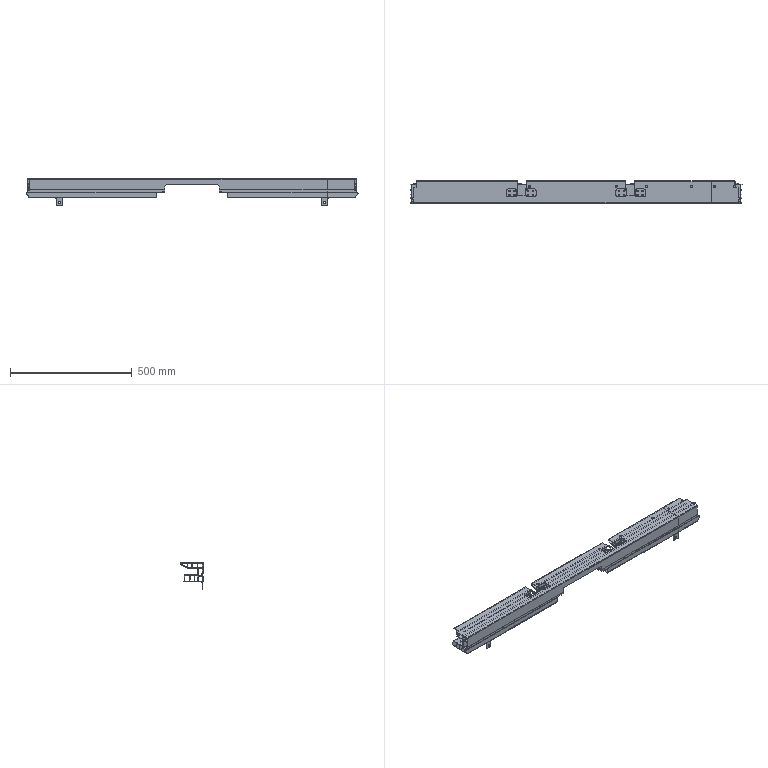NC program | NX | posted with a generic post | part box 1365 x 90.95 x 108.501 mm
Lines 11426 to 12338 of 22311:
(ZLEVEL_PROFILE_1 , TOOL : D8R0.5)
N22790 T08 M6
N22792 G54
N22794 G17 G0 G90 X562.492 Y46.775 B0. C0. S6000 M3
N22796 G43 Z30. H8
N22798 Z-23.6
N22800 G94 G1 Z-25.1 F1000.
N22802 X561.401 Y46.146
N22804 G3 X561.001 Y45.453 R0.8
N22806 G1 X561. Y41.818 F2500.
N22808 Y41.796 Z-25.2
N22810 X561.001 Y41.841
N22812 Y45.032
N22814 X561.002 Y45.475
N22816 Y45.497 Z-25.3
N22818 X561.001 Y41.841
N22820 X561. Y41.773
N22822 X560.999 Y41.75 Z-25.4
N22824 X561.002 Y45.519
N22826 Y45.542 Z-25.5
N22828 X560.999 Y41.727
N22830 X561.007 Y41.704 Z-25.6
N22832 X561.002 Y42.173
N22834 Y45.175
N22836 X561.009 Y45.564
N22838 X561.017 Y45.586 Z-25.7
N22840 G2 X561.005 Y45.175 R3.19
N22842 G1 Y42.169
N22844 G2 X561.015 Y41.681 R38.7
N22846 G1 X561.022 Y41.658 Z-25.8
N22848 G3 X561.011 Y42.163 R5.079
N22850 G1 Y45.175
N22852 G3 X561.026 Y45.608 R2.979
N22854 G1 X561.035 Y45.631 Z-25.899
N22856 G2 X561.019 Y45.032 R6.056
N22858 G1 Y42.153
N22860 G2 X561.03 Y41.635 R5.599
N22862 G1 X561.042 Y41.612 Z-25.999
N22864 G3 X561.029 Y42.142 R5.498
N22866 G1 Y45.032
N22868 G3 X561.05 Y45.653 R4.702
N22870 G1 X561.068 Y45.675 Z-26.098
N22872 G2 X561.041 Y44.982 R5.854
N22874 G1 Y42.128
N22876 G2 X561.056 Y41.589 R5.193
N22878 G1 X561.07 Y41.566 Z-26.197
N22880 G3 X561.055 Y42.112 R5.345
N22882 G1 Y44.932
N22884 G3 X561.086 Y45.675 R5.114
N22886 G1 X561.099 Z-26.246
N22888 X561.107 Z-26.296
N22890 G2 X561.072 Y44.874 R5.56
N22892 G1 Y42.093
N22894 G2 X561.091 Y41.54 R4.815
N22896 G1 X561.112 Y41.514 Z-26.394
N22898 X561.091 Y42.24
N22900 Y44.883
N22902 G3 X561.128 Y45.675 R4.587
N22904 G1 X561.141 Z-26.443
N22906 X561.149 Z-26.492
N22908 G2 X561.132 Y45.032 R8.455
N22910 G1 X561.111 Y44.883
N22912 Y42.24
N22914 X561.134 Y41.489
N22916 X561.155 Y41.463 Z-26.589
N22918 G3 X561.135 Y42.022 R10.677
N22920 G1 Y44.882
N22922 G3 X561.171 Y45.675 R5.365
N22924 G1 X561.19 Z-26.637
N22926 X561.202 Z-26.685
N22928 G2 X561.16 Y44.882 R5.175
N22930 G1 Y42.24
N22932 X561.178 Y41.435
N22934 X561.207 Y41.392 Z-26.781
N22936 X561.187 Y42.24
N22938 Y44.871
N22940 G3 X561.232 Y45.675 R4.853
N22942 G1 X561.251 Z-26.829
N22944 X561.263 Z-26.877
N22946 G2 X561.217 Y44.87 R4.776
N22948 G1 Y41.929
N22950 X561.227 Y41.841
N22952 X561.24 Y41.442
N22954 X561.236 Y41.349
N22956 X561.266 Y41.307 Z-26.972
N22958 G3 X561.257 Y41.893 R4.71
N22960 G2 X561.248 Y42.111 R2.833
N22962 G1 Y44.869
N22964 G3 X561.296 Y45.675 R4.865
N22966 G1 X561.311 Z-27.019
N22968 X561.329 Z-27.066
N22970 G2 X561.301 Y44.97 R6.773
N22972 G1 X561.304 Y44.922
N22974 X561.282 Y44.879
N22976 Y41.856
N22978 G2 X561.298 Y41.264 R5.522
N22980 G1 X561.336 Y41.221 Z-27.159
N22982 G2 X561.318 Y42.24 R209.932
N22984 G1 Y44.878
N22986 X561.338 Y44.949
N22988 G3 X561.362 Y45.675 R9.107
N22990 G1 X561.387 Z-27.205
N22992 X561.404 Z-27.251
N22994 G2 X561.369 Y44.918 R6.766
N22996 G1 X561.356 Y44.852
N22998 Y42.24
N23000 G3 X561.376 Y41.18 R183.601
N23002 G1 X561.416 Y41.138 Z-27.343
N23004 G3 X561.395 Y41.73 R5.067
N23006 G1 Y44.851
N23008 X561.402 Y44.876
N23010 X561.408 Y44.924
N23012 G3 X561.445 Y45.675 R5.343
N23014 G1 X561.47 Z-27.388
N23016 X561.49 Z-27.433
N23018 G2 X561.437 Y44.864 R4.5
N23020 G1 Y41.841
N23022 G2 X561.456 Y41.098 R11.859
N23024 G1 X561.5 Y41.243 Z-27.523
N23026 G3 X561.481 Y41.745 R4.037
N23028 G1 Y44.849
N23030 G3 X561.537 Y45.675 R4.2
N23032 G1 X561.55 Z-27.567
N23034 X561.583 Z-27.611
N23036 G2 X561.527 Y44.847 R3.997
N23038 G1 Y41.693
N23040 G2 X561.546 Y40.983 R4.483
N23042 G1 X561.593 Y40.921 Z-27.699
N23044 G3 X561.575 Y41.64 R4.285
N23046 G1 Y44.844
N23048 G3 X561.629 Y45.675 R4.101
N23050 G1 X561.655 Z-27.742
N23052 X561.678 Z-27.785
N23054 G2 X561.624 Y44.842 R4.557
N23056 G1 Y41.584
N23058 X561.639 Y41.442
N23060 X561.64 Y40.859
N23062 X561.693 Y40.798 Z-27.87
N23064 X561.681 Y41.499
N23066 X561.676 Y41.526
N23068 Y44.839
N23070 G3 X561.731 Y45.675 R4.263
N23072 G1 X561.758 Z-27.912
N23074 X561.783 Z-27.954
N23076 G2 X561.729 Y44.837 R4.285
N23078 G1 Y41.466
N23080 G2 X561.749 Y40.737 R8.083
N23082 G1 X561.805 Y40.678 Z-28.037
N23084 G3 X561.784 Y41.301 R12.709
N23086 G1 Y44.834
N23088 G3 X561.834 Y45.675 R4.69
N23090 G1 X561.866 Z-28.078
N23092 X561.894 Z-28.119
N23094 G2 X561.841 Y44.844 R4.71
N23096 G1 Y41.308
N23098 X561.851 Y41.178
N23100 X561.863 Y40.645
N23102 X561.862 Y40.613
N23104 X561.921 Y40.538 Z-28.199
N23106 X561.9 Y41.442
N23108 Y44.828
N23110 G3 X561.957 Y45.675 R4.443
N23112 G1 X561.992 Z-28.238
N23114 X562.018 Z-28.278
N23116 G2 X561.96 Y44.822 R4.391
N23118 G1 Y41.107
N23120 X561.974 Y41.043
N23122 X561.982 Y40.463
N23124 X562.045 Y40.39 Z-28.355
N23126 X562.023 Y41.442
N23128 Y44.826
N23130 G3 X562.082 Y45.675 R4.391
N23132 G1 X562.113 Z-28.393
N23134 X562.148 Z-28.431
N23136 G2 X562.086 Y44.82 R4.09
N23138 G1 Y41.043
N23140 X562.11 Y40.318
N23142 X562.174 Y40.248 Z-28.506
N23144 G3 X562.152 Y40.895 R4.075
N23146 G1 Y44.813
N23148 G3 X562.212 Y45.675 R4.148
N23150 G1 X562.248 Z-28.542
N23152 X562.28 Z-28.579
N23154 G2 X562.219 Y44.795 R4.613
N23156 G1 Y40.906
N23158 X562.224 Y40.881
N23160 X562.243 Y40.168
N23162 X562.31 Y40.083 Z-28.65
N23164 X562.303 Y40.645
N23166 X562.287 Y40.745
N23168 Y44.79
N23170 G3 X562.352 Y45.675 R4.359
N23172 G1 X562.391 Z-28.685
N23174 X562.422 Z-28.72
N23176 G2 X562.357 Y44.785 R4.493
N23178 G1 Y40.667
N23180 X562.37 Y40.645
N23182 X562.381 Y39.999
N23184 X562.453 Y39.918 Z-28.788
N23186 X562.429 Y40.677
N23188 Y44.806
N23190 G3 X562.496 Y45.675 R4.081
N23192 G1 X562.528 Z-28.821
N23194 X562.57 Z-28.855
N23196 G2 X562.501 Y44.8 R3.85
N23198 G1 Y40.507
N23200 G2 X562.525 Y39.837 R20.53
N23202 G1 X562.6 Y39.748 Z-28.92
N23204 G3 X562.576 Y40.424 R3.584
N23206 G1 Y44.778
N23208 G3 X562.644 Y45.675 R4.596
N23210 G1 X562.689 Z-28.951
N23212 X562.727 Z-28.983
N23214 X562.683 Y44.906
N23216 X562.651 Y44.756
N23218 Y40.433
N23220 X562.678 Y39.657
N23222 X562.758 Y39.565 Z-29.044
N23224 G3 X562.728 Y40.255 R3.732
N23226 G1 Y44.754
N23228 X562.765 Y44.904
N23230 X562.808 Y45.675
N23232 X562.846 Z-29.074
N23234 X562.887 Z-29.104
N23236 X562.845 Y44.902
N23238 X562.806 Y44.752
N23240 Y40.246
N23242 G2 X562.836 Y39.477 R16.227
N23244 G1 X562.914 Y39.384 Z-29.162
N23246 X562.916 Y39.448
N23248 X562.893 Y40.131
N23250 X562.885 Y40.166
N23252 Y44.767
N23254 X562.922 Y44.9
N23256 X562.964 Y45.675
N23258 X563. Z-29.19
N23260 X563.04 Z-29.218
N23262 X562.987 Y44.832
N23264 X562.965 Y44.765
N23266 Y39.991
N23268 G2 X562.994 Y39.292 R3.373
N23270 G1 X563.077 Y39.196 Z-29.272
N23272 X563.062 Y39.847
N23274 X563.047 Y39.983
N23276 Y44.743
N23278 G3 X563.128 Y45.675 R4.156
N23280 G1 X563.176 Z-29.298
N23282 X563.213 Z-29.324
N23284 X563.148 Y44.786
N23286 X563.129 Y44.721
N23288 Y39.885
N23290 X563.138 Y39.851
N23292 X563.162 Y39.102
N23294 X563.245 Y39.005 Z-29.375
N23296 X563.226 Y39.745
N23298 X563.213 Y39.779
N23300 Y44.736
N23302 X563.229 Y44.788
N23304 X563.295 Y45.676
N23306 X563.34 Z-29.399
N23308 X563.374 Z-29.423
N23310 X563.308 Y44.79
N23312 X563.297 Y44.764
N23314 Y39.714
N23316 X563.312 Y39.642
N23318 X563.331 Y39.049
N23320 X563.329 Y38.906
N23322 X563.413 Y38.811 Z-29.47
N23324 X563.392 Y39.563
N23326 X563.382 Y39.593
N23328 Y44.815
N23330 X563.457 Y45.676
N23332 X563.503 Z-29.493
N23334 X563.544 Z-29.515
N23336 G2 X563.469 Y44.815 R3.844
N23338 G1 Y39.508
N23340 X563.48 Y39.479
N23342 X563.507 Y38.707
N23344 X563.598 Y38.602 Z-29.558
N23346 X563.556 Y39.448
N23348 Y44.814
N23350 X563.574 Y44.868
N23352 X563.627 Y45.676
N23354 X563.671 Z-29.579
N23356 X563.707 Z-29.599
N23358 X563.644 Y44.848
N23360 Y39.238
N23362 G2 X563.688 Y38.497 R2.598
N23364 G1 X563.777 Y38.396 Z-29.638
N23366 X563.733 Y39.256
N23368 Y44.927
N23370 X563.747 Y44.956
N23372 X563.783 Y45.676
N23374 X563.824 Y45.677 Z-29.657
N23376 X563.863 Y45.678 Z-29.676
N23378 X563.823 Y45.175
N23380 Y39.145
N23382 X563.842 Y39.049
N23384 X563.868 Y38.296
N23386 X563.962 Y38.188 Z-29.711
N23388 X563.934 Y38.992
N23390 X563.914 Y39.033
N23392 Y45.177
N23394 X563.944 Y45.681
N23396 X563.979 Y45.682 Z-29.727
N23398 X564.024 Y45.683 Z-29.744
N23400 X564.005 Y45.18
N23402 Y38.962
N23404 X564.03 Y38.897
N23406 X564.058 Y38.077
N23408 X564.151 Y37.974 Z-29.775
N23410 X564.12 Y38.808
N23412 X564.096 Y38.853
N23414 Y45.184
N23416 X564.12 Y45.685
N23418 X564.166 Y45.686 Z-29.79
N23420 X564.211 Y45.688 Z-29.804
N23422 X564.201 Y45.21
N23424 X564.187 Y45.18
N23426 Y38.763
N23428 G2 X564.248 Y37.868 R1.827
N23430 G1 X564.34 Y37.76 Z-29.831
N23432 X564.278 Y38.69
N23434 Y45.032
N23436 X564.317 Y45.692
N23438 X564.355 Y45.694 Z-29.843
N23440 X564.414 Y45.696 Z-29.855
N23442 X564.368 Y45.032
N23444 Y38.431
N23446 G2 X564.389 Y37.047 R3.957
N23448 G1 X564.468 Y37.231 Z-29.866
N23450 X564.536 Y37.416 Z-29.878
N23452 X564.537 Y37.591
N23454 X564.459 Y38.331
N23456 Y45.197
N23458 X564.503 Y45.7
N23460 X564.546 Y45.702 Z-29.889
N23462 X564.592 Y45.704 Z-29.9
N23464 X564.557 Y45.201
N23466 Y38.422
N23468 X564.592 Y38.312
N23470 X564.643 Y37.426
N23472 G3 X565.082 Y36.757 R0.8
N23474 G1 X566.109 Y36.24
N23476 Z-28.4
N23478 G0 Z30.
N23480 X527.525 Y40.504
N23482 Z-23.6
N23484 G1 Z-25.1 F1000.
N23486 X528.601 Y41.125
N23488 G3 X529.001 Y41.818 R0.8
N23490 G1 Y45.454 F2500.
N23492 Y45.477 Z-25.2
N23494 Y41.841
N23496 X529.002 Y41.796
N23498 Y41.773 Z-25.3
N23500 X529.001 Y41.841
N23502 Y45.5
N23504 Y45.523 Z-25.4
N23506 Y41.841
N23508 X529.002 Y41.75
N23510 Y41.727 Z-25.5
N23512 X529. Y41.841
N23514 X529.001 Y45.032
N23516 X529. Y45.546
N23518 X528.992 Y45.569 Z-25.6
N23520 X529. Y45.175
N23522 Y42.173
N23524 X528.996 Y41.705
N23526 X528.989 Y41.682 Z-25.7
N23528 G2 X528.996 Y42.169 R4.46
N23530 G1 Y45.175
N23532 G2 X528.984 Y45.592 R3.342
N23534 G1 X528.974 Y45.616 Z-25.8
N23536 G3 X528.991 Y45.175 R3.443
N23538 G1 Y42.163
N23540 G3 X528.98 Y41.658 R5.147
N23542 G1 X528.97 Y41.635 Z-25.899
N23544 X528.983 Y42.153
N23546 Y45.175
N23548 G2 X528.961 Y45.639 R3.689
N23550 G1 X528.946 Y45.662 Z-25.999
N23552 G3 X528.973 Y45.175 R2.763
N23554 G1 Y42.142
N23556 G3 X528.958 Y41.612 R6.887
N23558 G1 X528.946 Y41.59 Z-26.098
N23560 G2 X528.961 Y42.128 R5.637
N23562 G1 Y44.982
N23564 G2 X528.93 Y45.675 R6.171
N23566 G1 X528.916 Z-26.148
N23568 X528.91 Z-26.197
N23570 G3 X528.947 Y44.932 R5.753
N23572 G1 Y42.112
N23574 G3 X528.932 Y41.566 R5.228
N23576 G1 X528.912 Y41.541 Z-26.296
N23578 G2 X528.93 Y42.093 R4.719
N23580 G1 Y44.915
N23582 G2 X528.89 Y45.675 R5.026
N23584 G1 X528.876 Z-26.345
N23586 X528.871 Z-26.394
N23588 G3 X528.911 Y44.898 R4.88
N23590 G1 Y42.24
N23592 G3 X528.89 Y41.515 R13.961
N23594 G1 X528.869 Y41.489 Z-26.492
N23596 X528.89 Y42.24
N23598 Y44.895
N23600 G2 X528.851 Y45.675 R4.893
N23602 G1 X528.837 Z-26.54
N23604 X528.829 Z-26.589
N23606 G3 X528.86 Y44.906 R7.665
N23608 G1 X528.867 Y44.892
N23610 Y42.022
N23612 G3 X528.847 Y41.463 R6.362
N23614 G1 X528.825 Y41.435 Z-26.685
N23616 X528.842 Y42.24
N23618 Y44.889
N23620 G2 X528.798 Y45.675 R5.194
N23622 G1 X528.779 Z-26.733
N23624 X528.768 Z-26.781
N23626 G3 X528.815 Y44.885 R4.678
N23628 G1 Y42.24
N23630 X528.796 Y41.392
N23632 X528.766 Y41.349 Z-26.877
N23634 X528.763 Y41.442
N23636 X528.775 Y41.841
N23638 X528.785 Y41.929
N23640 Y44.881
N23642 G2 X528.738 Y45.675 R4.658
N23644 G1 X528.719 Z-26.924
N23646 X528.705 Z-26.972
N23648 G3 X528.753 Y44.877 R4.76
N23650 G1 Y42.108
N23652 G2 X528.745 Y41.889 R2.878
N23654 G3 X528.737 Y41.306 R4.732
N23656 G1 X528.704 Y41.263 Z-27.066
N23658 G2 X528.72 Y41.856 R5.625
N23660 G1 Y44.873
N23662 G2 X528.672 Y45.675 R4.543
N23664 G1 X528.656 Z-27.112
N23666 X528.639 Z-27.159
N23668 G3 X528.684 Y44.868 R4.806
N23670 G1 Y42.24
N23672 G3 X528.667 Y41.221 R855.745
N23674 G1 X528.626 Y41.179 Z-27.251
N23676 G2 X528.646 Y42.24 R854.206
N23678 G1 Y44.862
N23680 G2 X528.598 Y45.675 R4.787
N23682 G1 X528.573 Z-27.297
N23684 X528.557 Z-27.343
N23686 G3 X528.606 Y44.857 R4.671
N23688 G1 Y41.73
N23690 G3 X528.586 Y41.138 R5.243
N23692 G1 X528.547 Y41.097 Z-27.433
N23694 G2 X528.565 Y41.841 R12.386
N23696 G1 Y44.852
N23698 G2 X528.512 Y45.675 R4.821
N23700 G1 X528.492 Z-27.478
N23702 X528.465 Z-27.523
N23704 G3 X528.521 Y44.849 R4.197
N23706 G1 Y41.744
N23708 G3 X528.503 Y41.046 R5.936
N23710 G1 X528.457 Y40.983 Z-27.611
N23712 G2 X528.475 Y41.691 R4.546
N23714 G1 Y44.847
N23716 G2 X528.419 Y45.675 R3.995
N23718 G1 X528.399 Z-27.655
N23720 X528.373 Z-27.699
N23722 G3 X528.427 Y44.844 R4.101
N23724 G1 Y41.635
N23726 G3 X528.41 Y40.921 R4.298
N23728 G1 X528.362 Y40.859 Z-27.785
N23730 X528.364 Y41.442
N23732 X528.378 Y41.577
N23734 Y44.842
N23736 G2 X528.324 Y45.675 R4.557
N23738 G1 X528.295 Z-27.828
N23740 X528.271 Z-27.87
N23742 G3 X528.326 Y44.839 R4.263
N23744 G1 Y41.517
N23746 X528.321 Y41.489
N23748 X528.31 Y40.798
N23750 X528.254 Y40.738 Z-27.954
N23752 X528.269 Y41.429
N23754 X528.273 Y41.442
N23756 Y44.837
N23758 G2 X528.219 Y45.675 R4.285
N23760 G1 X528.193 Z-27.996
N23762 X528.168 Z-28.037
N23764 G3 X528.217 Y44.834 R4.69
N23766 G1 Y41.301
N23768 G3 X528.198 Y40.679 R4.932
N23770 G1 X528.142 Y40.614 Z-28.119
N23772 X528.151 Y41.159
N23774 X528.161 Y41.238
N23776 Y44.844
N23778 G2 X528.108 Y45.675 R4.71
N23780 G1 X528.072 Z-28.159
N23782 X528.045 Z-28.199
N23784 G3 X528.102 Y44.828 R4.443
N23786 G1 Y41.442
N23788 X528.082 Y40.539
N23790 X528.021 Y40.464 Z-28.278
N23792 X528.028 Y41.043
N23794 X528.041 Y41.107
N23796 Y44.822
N23798 G2 X527.983 Y45.675 R4.391
N23800 G1 X527.949 Z-28.316
N23802 X527.92 Z-28.355
N23804 G3 X527.979 Y44.826 R4.391
N23806 G1 Y41.442
N23808 X527.958 Y40.391
N23810 X527.893 Y40.319 Z-28.431
N23812 X527.915 Y41.04
N23814 Y44.82
N23816 G2 X527.854 Y45.675 R4.09
N23818 G1 X527.827 Z-28.468
N23820 X527.79 Z-28.506
N23822 G3 X527.85 Y44.813 R4.147
N23824 G1 Y40.896
N23826 G3 X527.829 Y40.248 R4.321
N23828 G1 X527.764 Y40.169 Z-28.579
N23830 X527.778 Y40.871
N23832 X527.783 Y40.898
N23834 Y44.795
N23836 G2 X527.722 Y45.675 R4.612
N23838 G1 X527.681 Z-28.614
N23840 X527.65 Z-28.65
N23842 G3 X527.715 Y44.79 R4.357
N23844 G1 Y40.745
N23846 X527.701 Y40.645
N23848 X527.694 Y40.084
N23850 X527.623 Y40. Z-28.72
N23852 X527.645 Y40.667
N23854 Y44.785
N23856 G2 X527.58 Y45.675 R4.49
N23858 G1 X527.542 Z-28.754
N23860 X527.506 Z-28.788
N23862 G3 X527.573 Y44.806 R4.073
N23864 G1 Y40.645
N23866 X527.551 Y39.919
N23868 X527.479 Y39.839 Z-28.855
N23870 G2 X527.5 Y40.507 R4.267
N23872 G1 Y44.8
N23874 G2 X527.432 Y45.675 R3.835
N23876 G1 X527.395 Z-28.887
N23878 X527.358 Z-28.92
N23880 G3 X527.426 Y44.778 R4.555
N23882 G1 Y40.424
N23884 X527.402 Y39.847
N23886 X527.404 Y39.749
N23888 X527.327 Y39.659 Z-28.983
N23890 X527.351 Y40.417
N23892 Y44.749
N23894 X527.319 Y44.903
N23896 X527.275 Y45.675
N23898 X527.234 Z-29.013
N23900 X527.194 Z-29.044
N23902 X527.237 Y44.9
N23904 X527.274 Y44.747
N23906 Y40.294
N23908 X527.267 Y40.251
N23910 X527.247 Y39.567
N23912 X527.168 Y39.479 Z-29.104
N23914 X527.184 Y40.167
N23916 X527.196 Y40.234
N23918 Y44.76
N23920 X527.157 Y44.898
N23922 X527.116 Y45.675
N23924 X527.083 Z-29.133
N23926 X527.04 Z-29.162
N23928 X527.079 Y44.896
N23930 X527.117 Y44.758
N23932 Y40.129
N23934 X527.103 Y40.088
N23936 X527.09 Y39.387
N23938 X527.011 Y39.294 Z-29.218
N23940 X527.025 Y40.012
N23942 X527.036 Y40.051
N23944 Y44.756
N23946 X527.015 Y44.824
N23948 X526.964 Y45.675
N23950 X526.916 Z-29.245
N23952 X526.877 Z-29.272
N23954 G3 X526.955 Y44.736 R4.012
N23956 G1 Y39.977
N23958 X526.941 Y39.847
N23960 X526.927 Y39.199
N23962 X526.843 Y39.104 Z-29.324
N23964 X526.873 Y39.847
N23966 Y44.725
N23968 G2 X526.793 Y45.675 R3.874
N23970 G1 X526.749 Z-29.349
N23972 X526.712 Z-29.375
N23974 X526.769 Y44.775
N23976 X526.789 Y44.714
N23978 Y39.764
N23980 X526.774 Y39.719
N23982 X526.76 Y39.008
N23984 X526.676 Y38.91 Z-29.423
N23986 X526.689 Y39.617
N23988 X526.705 Y39.69
N23990 Y44.762
N23992 G2 X526.634 Y45.676 R3.803
N23994 G1 X526.59 Z-29.447
N23996 X526.554 Z-29.47
N23998 G3 X526.619 Y44.771 R4.432
N24000 G1 Y39.587
N24002 X526.608 Y39.518
N24004 X526.592 Y38.815
N24006 X526.499 Y38.71 Z-29.515
N24008 X526.522 Y39.448
N24010 X526.533 Y39.489
N24012 Y44.762
N24014 X526.516 Y44.822
N24016 X526.466 Y45.676
N24018 X526.423 Z-29.537
N24020 X526.382 Z-29.558
N24022 X526.432 Y44.765
N24024 X526.446 Y44.742
N24026 Y39.421
N24028 X526.408 Y38.606
N24030 X526.318 Y38.501 Z-29.599
N24032 G2 X526.358 Y39.238 R2.768
N24034 G1 Y44.76
N24036 X526.344 Y44.783
N24038 X526.302 Y45.676
N24040 X526.262 Z-29.619
N24042 X526.225 Z-29.638
N24044 X526.268 Y44.814
N24046 Y39.206
N24048 X526.255 Y39.178
N24050 X526.229 Y38.4
N24052 X526.138 Y38.301 Z-29.676
N24054 X526.165 Y39.08
N24056 X526.179 Y39.124
N24058 Y44.949
N24060 X526.144 Y45.678
N24062 X526.109 Y45.679 Z-29.693
N24064 X526.061 Y45.68 Z-29.711
N24066 X526.088 Y45.177
N24068 Y39.014
N24070 X526.066 Y38.965
N24072 X526.044 Y38.252
N24074 X526.045 Y38.194
N24076 X525.949 Y38.083 Z-29.744
N24078 X525.97 Y38.865
N24080 X525.997 Y38.941
N24082 Y45.18
N24084 X525.979 Y45.683
N24086 X525.929 Y45.684 Z-29.76
N24088 X525.883 Y45.685 Z-29.775
N24090 X525.906 Y45.184
N24092 Y38.824
N24094 X525.881 Y38.771
N24096 X525.856 Y37.979
N24098 X525.76 Y37.875 Z-29.804
N24100 G2 X525.814 Y38.728 R1.864
N24102 G1 Y45.181
N24104 X525.801 Y45.212
N24106 X525.79 Y45.688
N24108 X525.742 Y45.69 Z-29.817
N24110 X525.685 Y45.692 Z-29.831
N24112 X525.724 Y45.032
N24114 Y38.651
N24116 X525.668 Y37.767
N24118 X525.65 Y37.583 Z-29.836
N24120 X525.643 Y37.398 Z-29.84
N24122 X525.639 Y37.212 Z-29.845
N24124 X525.645 Y37.027 Z-29.85
N24126 X525.667 Y36.846 Z-29.855
N24128 X525.653 Y36.903
N24130 X525.575 Y38.252
N24132 X525.633 Y38.431
N24134 Y45.032
N24136 X525.587 Y45.696
N24138 X525.555 Y45.698 Z-29.866
N24140 X525.498 Y45.7 Z-29.878
N24142 X525.543 Y45.197
N24144 Y38.33
N24146 X525.473 Y37.563
N24148 X525.476 Y37.408
N24150 X525.368 Y37.435 Z-29.9
N24152 X525.409 Y38.267
N24154 X525.444 Y38.381
N24156 Y45.201
N24158 X525.408 Y45.704
N24160 G3 X524.959 Y46.366 R0.8
N24162 G1 X523.936 Y46.862
N24164 Z-28.4
N24166 G0 Z30.
N24168 X-527.508 Y46.775
N24170 Z-23.6
N24172 G1 Z-25.1 F1000.
N24174 X-528.599 Y46.146
N24176 G3 X-528.999 Y45.453 R0.8
N24178 G1 X-529. Y41.818 F2500.
N24180 Y41.796 Z-25.2
N24182 X-528.999 Y41.841
N24184 Y45.032
N24186 X-528.998 Y45.475
N24188 Y45.497 Z-25.3
N24190 X-528.999 Y41.841
N24192 X-529. Y41.773
N24194 X-529.001 Y41.75 Z-25.4
N24196 X-528.998 Y45.519
N24198 Y45.542 Z-25.5
N24200 X-529.001 Y41.727
N24202 X-528.993 Y41.704 Z-25.6
N24204 X-528.998 Y42.173
N24206 Y45.175
N24208 X-528.991 Y45.564
N24210 X-528.983 Y45.586 Z-25.7
N24212 G2 X-528.995 Y45.175 R3.19
N24214 G1 Y42.169
N24216 G2 X-528.985 Y41.681 R38.698
N24218 G1 X-528.978 Y41.658 Z-25.8
N24220 G3 X-528.989 Y42.163 R5.079
N24222 G1 Y45.175
N24224 G3 X-528.974 Y45.608 R2.979
N24226 G1 X-528.965 Y45.631 Z-25.899
N24228 G2 X-528.981 Y45.032 R6.056
N24230 G1 Y42.153
N24232 G2 X-528.97 Y41.635 R5.599
N24234 G1 X-528.958 Y41.612 Z-25.999
N24236 G3 X-528.971 Y42.142 R5.498
N24238 G1 Y45.032
N24240 G3 X-528.95 Y45.653 R4.702
N24242 G1 X-528.932 Y45.675 Z-26.098
N24244 G2 X-528.959 Y44.982 R5.854
N24246 G1 Y42.128
N24248 G2 X-528.944 Y41.589 R5.193
N24250 G1 X-528.93 Y41.566 Z-26.197
N24252 G3 X-528.945 Y42.112 R5.345
N24254 G1 Y44.932
N24256 G3 X-528.914 Y45.675 R5.114
N24258 G1 X-528.901 Z-26.246
N24260 X-528.893 Z-26.296
N24262 G2 X-528.928 Y44.874 R5.56
N24264 G1 Y42.093
N24266 G2 X-528.909 Y41.54 R4.815
N24268 G1 X-528.888 Y41.514 Z-26.394
N24270 X-528.909 Y42.24
N24272 Y44.883
N24274 G3 X-528.872 Y45.675 R4.587
N24276 G1 X-528.859 Z-26.443
N24278 X-528.851 Z-26.492
N24280 G2 X-528.868 Y45.032 R8.455
N24282 G1 X-528.889 Y44.883
N24284 Y42.24
N24286 X-528.866 Y41.489
N24288 X-528.845 Y41.463 Z-26.589
N24290 G3 X-528.865 Y42.022 R10.677
N24292 G1 Y44.882
N24294 G3 X-528.829 Y45.675 R5.364
N24296 G1 X-528.81 Z-26.637
N24298 X-528.798 Z-26.685
N24300 G2 X-528.84 Y44.882 R5.175
N24302 G1 Y42.24
N24304 X-528.822 Y41.435
N24306 X-528.793 Y41.392 Z-26.781
N24308 X-528.813 Y42.24
N24310 Y44.871
N24312 G3 X-528.768 Y45.675 R4.853
N24314 G1 X-528.749 Z-26.829
N24316 X-528.737 Z-26.877
N24318 G2 X-528.783 Y44.87 R4.776
N24320 G1 Y41.929
N24322 X-528.773 Y41.841
N24324 X-528.76 Y41.442
N24326 X-528.764 Y41.349
N24328 X-528.734 Y41.307 Z-26.972
N24330 G3 X-528.743 Y41.893 R4.71
N24332 G2 X-528.752 Y42.111 R2.833
N24334 G1 Y44.869
N24336 G3 X-528.704 Y45.675 R4.865
N24338 G1 X-528.689 Z-27.019
N24340 X-528.671 Z-27.066
N24342 G2 X-528.699 Y44.97 R6.773
N24344 G1 X-528.696 Y44.922
N24346 X-528.718 Y44.879
N24348 Y41.856
N24350 G2 X-528.702 Y41.264 R5.522
N24352 G1 X-528.664 Y41.221 Z-27.159
N24354 G2 X-528.682 Y42.24 R209.935
N24356 G1 Y44.878
N24358 X-528.662 Y44.949
N24360 G3 X-528.638 Y45.675 R9.107
N24362 G1 X-528.613 Z-27.205
N24364 X-528.596 Z-27.251
N24366 G2 X-528.631 Y44.918 R6.766
N24368 G1 X-528.644 Y44.852
N24370 Y42.24
N24372 G3 X-528.624 Y41.18 R183.602
N24374 G1 X-528.584 Y41.138 Z-27.343
N24376 G3 X-528.605 Y41.73 R5.067
N24378 G1 Y44.851
N24380 X-528.598 Y44.876
N24382 X-528.592 Y44.924
N24384 G3 X-528.555 Y45.675 R5.343
N24386 G1 X-528.53 Z-27.388
N24388 X-528.51 Z-27.433
N24390 G2 X-528.563 Y44.864 R4.5
N24392 G1 Y41.841
N24394 G2 X-528.544 Y41.098 R11.859
N24396 G1 X-528.5 Y41.243 Z-27.523
N24398 G3 X-528.519 Y41.745 R4.038
N24400 G1 Y44.849
N24402 G3 X-528.463 Y45.675 R4.2
N24404 G1 X-528.45 Z-27.567
N24406 X-528.417 Z-27.611
N24408 G2 X-528.473 Y44.847 R3.997
N24410 G1 Y41.693
N24412 G2 X-528.454 Y40.983 R4.483
N24414 G1 X-528.407 Y40.921 Z-27.699
N24416 G3 X-528.425 Y41.64 R4.285
N24418 G1 Y44.844
N24420 G3 X-528.371 Y45.675 R4.101
N24422 G1 X-528.345 Z-27.742
N24424 X-528.322 Z-27.785
N24426 G2 X-528.376 Y44.842 R4.557
N24428 G1 Y41.584
N24430 X-528.361 Y41.442
N24432 X-528.36 Y40.859
N24434 X-528.307 Y40.798 Z-27.87
N24436 X-528.319 Y41.499
N24438 X-528.324 Y41.526
N24440 Y44.839
N24442 G3 X-528.269 Y45.675 R4.263
N24444 G1 X-528.242 Z-27.912
N24446 X-528.217 Z-27.954
N24448 G2 X-528.271 Y44.837 R4.285
N24450 G1 Y41.466
N24452 G2 X-528.251 Y40.737 R8.083
N24454 G1 X-528.195 Y40.678 Z-28.037
N24456 G3 X-528.216 Y41.301 R12.709
N24458 G1 Y44.834
N24460 G3 X-528.166 Y45.675 R4.69
N24462 G1 X-528.134 Z-28.078
N24464 X-528.106 Z-28.119
N24466 G2 X-528.159 Y44.844 R4.71
N24468 G1 Y41.308
N24470 X-528.149 Y41.178
N24472 X-528.137 Y40.645
N24474 X-528.138 Y40.613
N24476 X-528.079 Y40.538 Z-28.199
N24478 X-528.1 Y41.442
N24480 Y44.828
N24482 G3 X-528.043 Y45.675 R4.443
N24484 G1 X-528.008 Z-28.238
N24486 X-527.982 Z-28.278
N24488 G2 X-528.04 Y44.822 R4.391
N24490 G1 Y41.107
N24492 X-528.026 Y41.043
N24494 X-528.018 Y40.463
N24496 X-527.955 Y40.39 Z-28.355
N24498 X-527.977 Y41.442
N24500 Y44.826
N24502 G3 X-527.918 Y45.675 R4.391
N24504 G1 X-527.887 Z-28.393
N24506 X-527.852 Z-28.431
N24508 G2 X-527.914 Y44.82 R4.09
N24510 G1 Y41.043
N24512 X-527.89 Y40.318
N24514 X-527.826 Y40.248 Z-28.506
N24516 G3 X-527.848 Y40.895 R4.075
N24518 G1 Y44.813
N24520 G3 X-527.788 Y45.675 R4.148
N24522 G1 X-527.752 Z-28.542
N24524 X-527.72 Z-28.579
N24526 G2 X-527.781 Y44.795 R4.613
N24528 G1 Y40.906
N24530 X-527.776 Y40.881
N24532 X-527.757 Y40.168
N24534 X-527.69 Y40.083 Z-28.65
N24536 X-527.697 Y40.645
N24538 X-527.713 Y40.745
N24540 Y44.79
N24542 G3 X-527.648 Y45.675 R4.359
N24544 G1 X-527.609 Z-28.685
N24546 X-527.578 Z-28.72
N24548 G2 X-527.643 Y44.785 R4.493
N24550 G1 Y40.667
N24552 X-527.63 Y40.645
N24554 X-527.619 Y39.999
N24556 X-527.547 Y39.918 Z-28.788
N24558 X-527.571 Y40.677
N24560 Y44.806
N24562 G3 X-527.504 Y45.675 R4.081
N24564 G1 X-527.472 Z-28.821
N24566 X-527.43 Z-28.855
N24568 G2 X-527.499 Y44.8 R3.85
N24570 G1 Y40.507
N24572 G2 X-527.475 Y39.837 R20.53
N24574 G1 X-527.4 Y39.748 Z-28.92
N24576 G3 X-527.424 Y40.424 R3.584
N24578 G1 Y44.778
N24580 G3 X-527.356 Y45.675 R4.596
N24582 G1 X-527.311 Z-28.951
N24584 X-527.273 Z-28.983
N24586 X-527.317 Y44.906
N24588 X-527.349 Y44.756
N24590 Y40.437
N24592 X-527.322 Y39.657
N24594 X-527.242 Y39.565 Z-29.044
N24596 G3 X-527.272 Y40.255 R3.732
N24598 G1 Y44.754
N24600 X-527.235 Y44.904
N24602 X-527.192 Y45.675
N24604 X-527.154 Z-29.074
N24606 X-527.113 Z-29.104
N24608 X-527.155 Y44.902